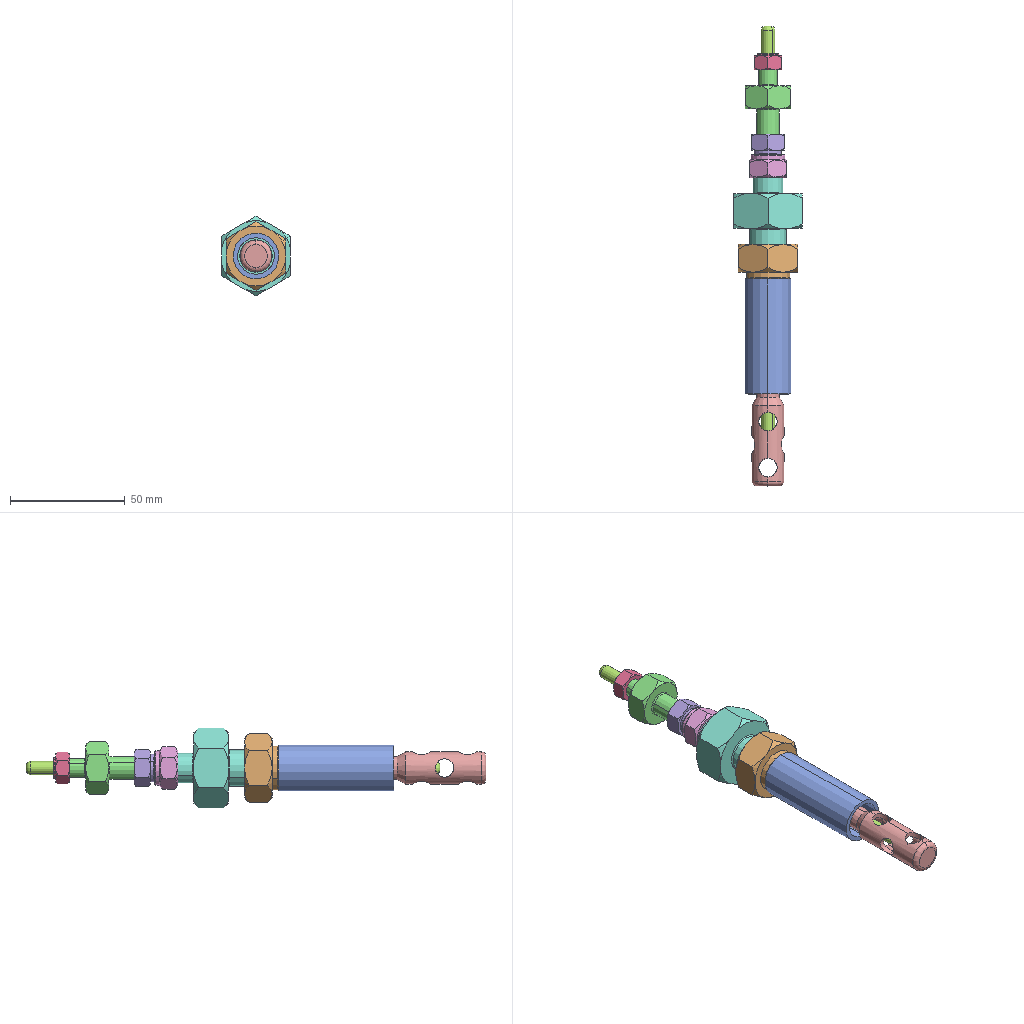Assembly | SolidWorks | 5 different items | 5 placed | box 30 x 200 x 35 mm
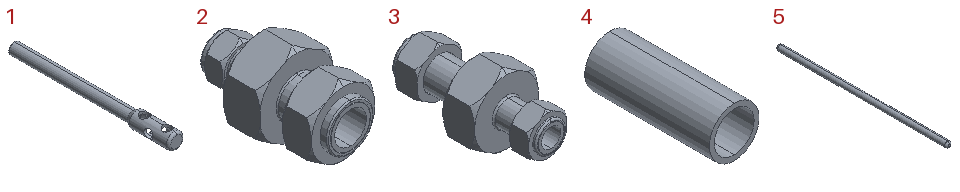Parts list (item | quantity | size | volume | features):
1 | x1 | 14 x 144 x 14 mm | 6707 mm3 | features ICE 7, Fillet 2, Extrusion 1, MoveFace 1, Revolution 1
2 | x1 | 30 x 54 x 34.641 mm | 18354 mm3 | features ICE 8, Fillet 3, Extrusion 1, RevCut 1
3 | x1 | 20 x 44 x 23.094 mm | 5151 mm3 | features ICE 8, Fillet 3, Extrusion 1, RevCut 1
4 | x1 | 20 x 50 x 20 mm | 5655 mm3 | features Extrusion 1
5 | x1 | 6 x 180 x 6 mm | 5062 mm3 | features Extrusion 1, Fillet 1
Mates (type | each side: item.copy, entity, surface, feature):
Coincident | 1.1 plane | assembly plane | 3 times
Concentric | 1.1 face cylinder Boss-Extrude1 | 4.1 face cylinder Boss-Extrude1
Concentric | 4.1 face cylinder Boss-Extrude1 | 5.1 face cylinder Boss-Extrude1
DistanceDim | 5.1 face plane Boss-Extrude1 | 1.1 face plane Boss-Extrude1
Concentric | 5.1 face cylinder Boss-Extrude1 | 2.1 face cylinder Boss-Extrude2
Concentric | 5.1 face cylinder Boss-Extrude1 | 3.1 face cylinder Boss-Extrude2
Coincident | 4.1 face plane Boss-Extrude1 | 2.1 face plane Boss-Extrude3
Parallel | 2.1 face plane Boss-Extrude1 | assembly plane
Parallel | 3.1 face plane Boss-Extrude1 | assembly plane
DistanceDim | 5.1 face plane Boss-Extrude1 | 3.1 face plane Boss-Extrude3